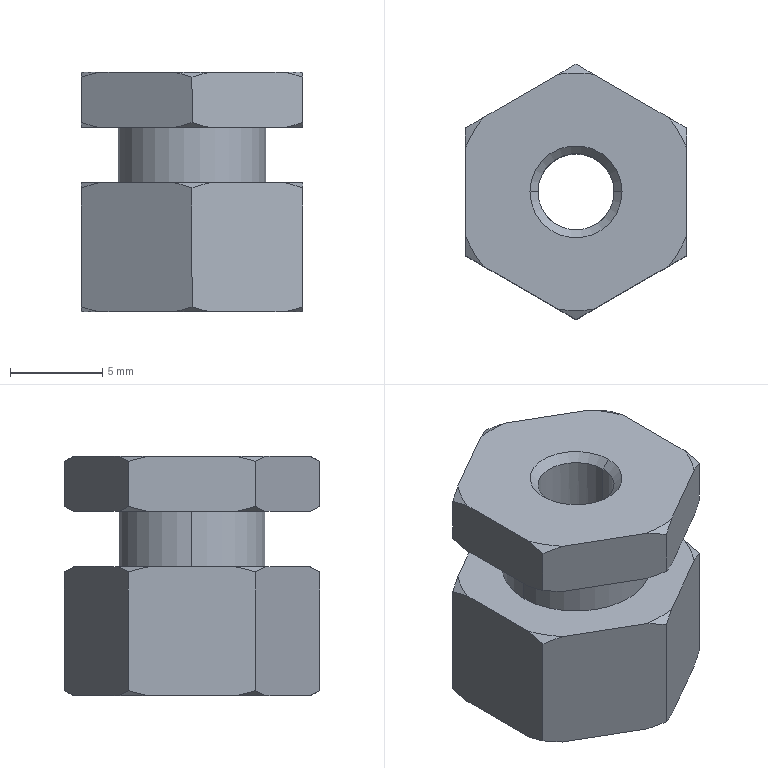Part | SolidWorks | features BaseBody 1 | 1 solid | 48 faces | box 12 x 13.856 x 13 mm | volume 1220 mm3 | cone 28 | plane 16 | cylinder 4 | commonest cylinder face diameters 4.134 x2 8 x2